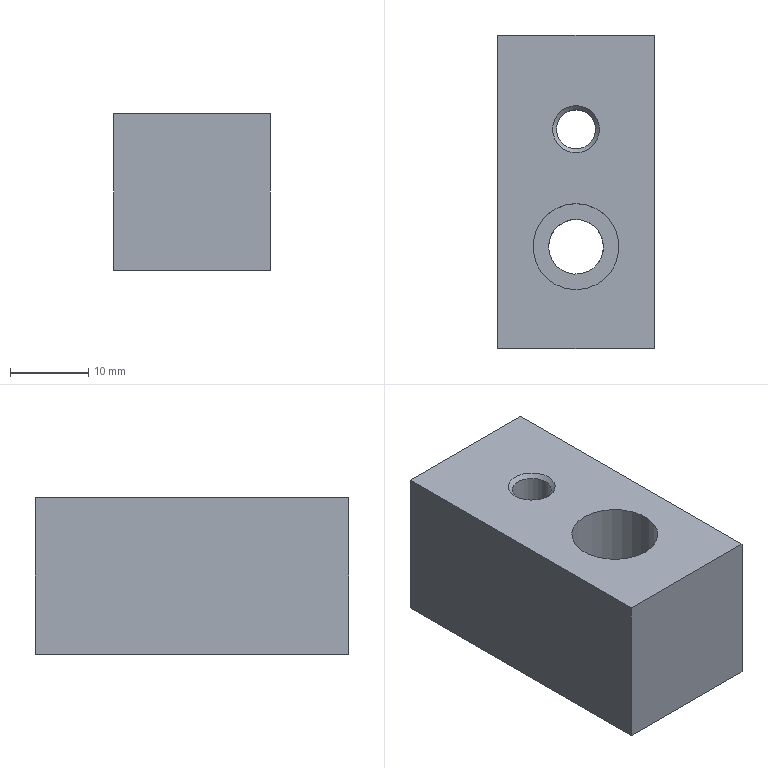Part | STEP file | gslz 2016.10.28-6_id18_x_t | 1 solid | 11 faces | box 20 x 40 x 20 mm | volume 14270 mm3 | plane 7 | cylinder 3 | cone 1 | commonest cylinder face diameters 5 x1 7 x1 11 x1
STEP:
#1=CARTESIAN_POINT('',(-127.2,158.,10.));
#2=VERTEX_POINT('',#1);
#3=CARTESIAN_POINT('',(-130.2,158.,10.));
#4=DIRECTION('',(0.,0.,-1.));
#5=DIRECTION('',(1.,0.,0.));
#6=AXIS2_PLACEMENT_3D('',#3,#4,#5);
#7=CIRCLE('',#6,3.);
#8=EDGE_CURVE('',#2,#2,#7,.T.);
#9=ORIENTED_EDGE('',*,*,#8,.T.);
#10=EDGE_LOOP('',(#9));
#11=FACE_BOUND('',#10,.T.);
#12=CARTESIAN_POINT('',(-140.2,130.,10.));
#13=VERTEX_POINT('',#12);
#14=CARTESIAN_POINT('',(-120.2,130.,10.));
#15=VERTEX_POINT('',#14);
#16=CARTESIAN_POINT('',(-138.2,130.,10.));
#17=DIRECTION('',(1.,0.,0.));
#18=VECTOR('',#17,1.);
#19=LINE('',#16,#18);
#20=EDGE_CURVE('',#13,#15,#19,.T.);
#21=ORIENTED_EDGE('',*,*,#20,.T.);
#22=CARTESIAN_POINT('',(-120.2,170.,10.));
#23=VERTEX_POINT('',#22);
#24=CARTESIAN_POINT('',(-120.2,130.,10.));
#25=DIRECTION('',(0.,1.,0.));
#26=VECTOR('',#25,1.);
#27=LINE('',#24,#26);
#28=EDGE_CURVE('',#15,#23,#27,.T.);
#29=ORIENTED_EDGE('',*,*,#28,.T.);
#30=CARTESIAN_POINT('',(-140.2,170.,10.));
#31=VERTEX_POINT('',#30);
#32=CARTESIAN_POINT('',(-122.2,170.,10.));
#33=DIRECTION('',(-1.,0.,0.));
#34=VECTOR('',#33,1.);
#35=LINE('',#32,#34);
#36=EDGE_CURVE('',#23,#31,#35,.T.);
#37=ORIENTED_EDGE('',*,*,#36,.T.);
#38=CARTESIAN_POINT('',(-140.2,160.,10.));
#39=DIRECTION('',(0.,-1.,0.));
#40=VECTOR('',#39,1.);
#41=LINE('',#38,#40);
#42=EDGE_CURVE('',#31,#13,#41,.T.);
#43=ORIENTED_EDGE('',*,*,#42,.T.);
#44=EDGE_LOOP('',(#21,#29,#37,#43));
#45=FACE_BOUND('',#44,.T.);
#46=CARTESIAN_POINT('',(-130.2,148.5,10.));
#47=VERTEX_POINT('',#46);
#48=CARTESIAN_POINT('',(-130.2,143.,10.));
#49=DIRECTION('',(0.,0.,1.));
#50=DIRECTION('',(0.,1.,0.));
#51=AXIS2_PLACEMENT_3D('',#48,#49,#50);
#52=CIRCLE('',#51,5.5);
#53=EDGE_CURVE('',#47,#47,#52,.T.);
#54=ORIENTED_EDGE('',*,*,#53,.F.);
#55=EDGE_LOOP('',(#54));
#56=FACE_BOUND('',#55,.T.);
#57=CARTESIAN_POINT('',(-138.2,130.,10.));
#58=DIRECTION('',(0.,0.,1.));
#59=DIRECTION('',(0.,-1.,0.));
#60=AXIS2_PLACEMENT_3D('',#57,#58,#59);
#61=PLANE('',#60);
#62=ADVANCED_FACE('',(#11,#45,#56),#61,.T.);
#63=CARTESIAN_POINT('',(-130.2,146.5,0.));
#64=VERTEX_POINT('',#63);
#65=CARTESIAN_POINT('',(-130.2,143.,0.));
#66=DIRECTION('',(0.,0.,1.));
#67=DIRECTION('',(0.,1.,0.));
#68=AXIS2_PLACEMENT_3D('',#65,#66,#67);
#69=CIRCLE('',#68,3.5);
#70=EDGE_CURVE('',#64,#64,#69,.T.);
#71=ORIENTED_EDGE('',*,*,#70,.F.);
#72=EDGE_LOOP('',(#71));
#73=FACE_BOUND('',#72,.T.);
#74=CARTESIAN_POINT('',(-130.2,148.5,0.));
#75=VERTEX_POINT('',#74);
#76=CARTESIAN_POINT('',(-130.2,143.,0.));
#77=DIRECTION('',(0.,0.,1.));
#78=DIRECTION('',(0.,1.,0.));
#79=AXIS2_PLACEMENT_3D('',#76,#77,#78);
#80=CIRCLE('',#79,5.5);
#81=EDGE_CURVE('',#75,#75,#80,.T.);
#82=ORIENTED_EDGE('',*,*,#81,.T.);
#83=EDGE_LOOP('',(#82));
#84=FACE_BOUND('',#83,.T.);
#85=CARTESIAN_POINT('',(-130.2,143.,0.));
#86=DIRECTION('',(0.,0.,1.));
#87=DIRECTION('',(0.,-1.,0.));
#88=AXIS2_PLACEMENT_3D('',#85,#86,#87);
#89=PLANE('',#88);
#90=ADVANCED_FACE('',(#73,#84),#89,.T.);
#91=CARTESIAN_POINT('',(-127.7,158.,9.5));
#92=VERTEX_POINT('',#91);
#93=CARTESIAN_POINT('',(-130.2,158.,9.5));
#94=DIRECTION('',(0.,0.,1.));
#95=DIRECTION('',(1.,0.,0.));
#96=AXIS2_PLACEMENT_3D('',#93,#94,#95);
#97=CIRCLE('',#96,2.5);
#98=EDGE_CURVE('',#92,#92,#97,.T.);
#99=ORIENTED_EDGE('',*,*,#98,.T.);
#100=EDGE_LOOP('',(#99));
#101=FACE_BOUND('',#100,.T.);
#102=CARTESIAN_POINT('',(-132.7,158.,-10.));
#103=VERTEX_POINT('',#102);
#104=CARTESIAN_POINT('',(-130.2,158.,-10.));
#105=DIRECTION('',(0.,0.,-1.));
#106=DIRECTION('',(-1.,0.,0.));
#107=AXIS2_PLACEMENT_3D('',#104,#105,#106);
#108=CIRCLE('',#107,2.5);
#109=EDGE_CURVE('',#103,#103,#108,.T.);
#110=ORIENTED_EDGE('',*,*,#109,.T.);
#111=EDGE_LOOP('',(#110));
#112=FACE_BOUND('',#111,.T.);
#113=CARTESIAN_POINT('',(-130.2,158.,24.));
#114=DIRECTION('',(0.,0.,-1.));
#115=DIRECTION('',(-1.,0.,0.));
#116=AXIS2_PLACEMENT_3D('',#113,#114,#115);
#117=CYLINDRICAL_SURFACE('',#116,2.5);
#118=ADVANCED_FACE('',(#101,#112),#117,.F.);
#119=ORIENTED_EDGE('',*,*,#36,.F.);
#120=CARTESIAN_POINT('',(-120.2,170.,-10.));
#121=VERTEX_POINT('',#120);
#122=CARTESIAN_POINT('',(-120.2,170.,8.));
#123=DIRECTION('',(0.,0.,1.));
#124=VECTOR('',#123,1.);
#125=LINE('',#122,#124);
#126=EDGE_CURVE('',#121,#23,#125,.T.);
#127=ORIENTED_EDGE('',*,*,#126,.F.);
#128=CARTESIAN_POINT('',(-140.2,170.,-10.));
#129=VERTEX_POINT('',#128);
#130=CARTESIAN_POINT('',(-122.2,170.,-10.));
#131=DIRECTION('',(-1.,0.,0.));
#132=VECTOR('',#131,1.);
#133=LINE('',#130,#132);
#134=EDGE_CURVE('',#121,#129,#133,.T.);
#135=ORIENTED_EDGE('',*,*,#134,.T.);
#136=CARTESIAN_POINT('',(-140.2,170.,8.));
#137=DIRECTION('',(0.,0.,1.));
#138=VECTOR('',#137,1.);
#139=LINE('',#136,#138);
#140=EDGE_CURVE('',#129,#31,#139,.T.);
#141=ORIENTED_EDGE('',*,*,#140,.T.);
#142=EDGE_LOOP('',(#119,#127,#135,#141));
#143=FACE_OUTER_BOUND('',#142,.T.);
#144=CARTESIAN_POINT('',(-122.2,170.,8.));
#145=DIRECTION('',(0.,-1.,0.));
#146=DIRECTION('',(0.,0.,-1.));
#147=AXIS2_PLACEMENT_3D('',#144,#145,#146);
#148=PLANE('',#147);
#149=ADVANCED_FACE('',(#143),#148,.F.);
#150=ORIENTED_EDGE('',*,*,#42,.F.);
#151=ORIENTED_EDGE('',*,*,#140,.F.);
#152=CARTESIAN_POINT('',(-140.2,130.,-10.));
#153=VERTEX_POINT('',#152);
#154=CARTESIAN_POINT('',(-140.2,160.,-10.));
#155=DIRECTION('',(0.,-1.,0.));
#156=VECTOR('',#155,1.);
#157=LINE('',#154,#156);
#158=EDGE_CURVE('',#129,#153,#157,.T.);
#159=ORIENTED_EDGE('',*,*,#158,.T.);
#160=CARTESIAN_POINT('',(-140.2,130.,8.));
#161=DIRECTION('',(0.,0.,1.));
#162=VECTOR('',#161,1.);
#163=LINE('',#160,#162);
#164=EDGE_CURVE('',#153,#13,#163,.T.);
#165=ORIENTED_EDGE('',*,*,#164,.T.);
#166=EDGE_LOOP('',(#150,#151,#159,#165));
#167=FACE_OUTER_BOUND('',#166,.T.);
#168=CARTESIAN_POINT('',(-140.2,160.,8.));
#169=DIRECTION('',(1.,0.,0.));
#170=DIRECTION('',(0.,0.,1.));
#171=AXIS2_PLACEMENT_3D('',#168,#169,#170);
#172=PLANE('',#171);
#173=ADVANCED_FACE('',(#167),#172,.F.);
#174=CARTESIAN_POINT('',(-120.2,130.,-10.));
#175=VERTEX_POINT('',#174);
#176=CARTESIAN_POINT('',(-138.2,130.,-10.));
#177=DIRECTION('',(1.,0.,0.));
#178=VECTOR('',#177,1.);
#179=LINE('',#176,#178);
#180=EDGE_CURVE('',#153,#175,#179,.T.);
#181=ORIENTED_EDGE('',*,*,#180,.T.);
#182=CARTESIAN_POINT('',(-120.2,130.,8.));
#183=DIRECTION('',(0.,0.,1.));
#184=VECTOR('',#183,1.);
#185=LINE('',#182,#184);
#186=EDGE_CURVE('',#175,#15,#185,.T.);
#187=ORIENTED_EDGE('',*,*,#186,.T.);
#188=ORIENTED_EDGE('',*,*,#20,.F.);
#189=ORIENTED_EDGE('',*,*,#164,.F.);
#190=EDGE_LOOP('',(#181,#187,#188,#189));
#191=FACE_OUTER_BOUND('',#190,.T.);
#192=CARTESIAN_POINT('',(-138.2,130.,8.));
#193=DIRECTION('',(0.,1.,0.));
#194=DIRECTION('',(0.,0.,1.));
#195=AXIS2_PLACEMENT_3D('',#192,#193,#194);
#196=PLANE('',#195);
#197=ADVANCED_FACE('',(#191),#196,.F.);
#198=ORIENTED_EDGE('',*,*,#28,.F.);
#199=ORIENTED_EDGE('',*,*,#186,.F.);
#200=CARTESIAN_POINT('',(-120.2,130.,-10.));
#201=DIRECTION('',(0.,1.,0.));
#202=VECTOR('',#201,1.);
#203=LINE('',#200,#202);
#204=EDGE_CURVE('',#175,#121,#203,.T.);
#205=ORIENTED_EDGE('',*,*,#204,.T.);
#206=ORIENTED_EDGE('',*,*,#126,.T.);
#207=EDGE_LOOP('',(#198,#199,#205,#206));
#208=FACE_OUTER_BOUND('',#207,.T.);
#209=CARTESIAN_POINT('',(-120.2,130.,8.));
#210=DIRECTION('',(-1.,0.,0.));
#211=DIRECTION('',(0.,0.,-1.));
#212=AXIS2_PLACEMENT_3D('',#209,#210,#211);
#213=PLANE('',#212);
#214=ADVANCED_FACE('',(#208),#213,.F.);
#215=CARTESIAN_POINT('',(-133.7,143.,-10.));
#216=VERTEX_POINT('',#215);
#217=CARTESIAN_POINT('',(-130.2,143.,-10.));
#218=DIRECTION('',(0.,0.,-1.));
#219=DIRECTION('',(-1.,0.,0.));
#220=AXIS2_PLACEMENT_3D('',#217,#218,#219);
#221=CIRCLE('',#220,3.5);
#222=EDGE_CURVE('',#216,#216,#221,.T.);
#223=ORIENTED_EDGE('',*,*,#222,.T.);
#224=EDGE_LOOP('',(#223));
#225=FACE_BOUND('',#224,.T.);
#226=ORIENTED_EDGE('',*,*,#70,.T.);
#227=EDGE_LOOP('',(#226));
#228=FACE_BOUND('',#227,.T.);
#229=CARTESIAN_POINT('',(-130.2,143.,24.));
#230=DIRECTION('',(0.,0.,-1.));
#231=DIRECTION('',(-1.,0.,0.));
#232=AXIS2_PLACEMENT_3D('',#229,#230,#231);
#233=CYLINDRICAL_SURFACE('',#232,3.5);
#234=ADVANCED_FACE('',(#225,#228),#233,.F.);
#235=ORIENTED_EDGE('',*,*,#222,.F.);
#236=EDGE_LOOP('',(#235));
#237=FACE_BOUND('',#236,.T.);
#238=ORIENTED_EDGE('',*,*,#204,.F.);
#239=ORIENTED_EDGE('',*,*,#180,.F.);
#240=ORIENTED_EDGE('',*,*,#158,.F.);
#241=ORIENTED_EDGE('',*,*,#134,.F.);
#242=EDGE_LOOP('',(#238,#239,#240,#241));
#243=FACE_BOUND('',#242,.T.);
#244=ORIENTED_EDGE('',*,*,#109,.F.);
#245=EDGE_LOOP('',(#244));
#246=FACE_BOUND('',#245,.T.);
#247=CARTESIAN_POINT('',(-130.2,130.,-10.));
#248=DIRECTION('',(0.,0.,-1.));
#249=DIRECTION('',(0.,1.,0.));
#250=AXIS2_PLACEMENT_3D('',#247,#248,#249);
#251=PLANE('',#250);
#252=ADVANCED_FACE('',(#237,#243,#246),#251,.T.);
#253=ORIENTED_EDGE('',*,*,#81,.F.);
#254=EDGE_LOOP('',(#253));
#255=FACE_BOUND('',#254,.T.);
#256=ORIENTED_EDGE('',*,*,#53,.T.);
#257=EDGE_LOOP('',(#256));
#258=FACE_BOUND('',#257,.T.);
#259=CARTESIAN_POINT('',(-130.2,143.,0.));
#260=DIRECTION('',(0.,0.,1.));
#261=DIRECTION('',(1.,0.,0.));
#262=AXIS2_PLACEMENT_3D('',#259,#260,#261);
#263=CYLINDRICAL_SURFACE('',#262,5.5);
#264=ADVANCED_FACE('',(#255,#258),#263,.F.);
#265=ORIENTED_EDGE('',*,*,#98,.F.);
#266=EDGE_LOOP('',(#265));
#267=FACE_BOUND('',#266,.T.);
#268=ORIENTED_EDGE('',*,*,#8,.F.);
#269=EDGE_LOOP('',(#268));
#270=FACE_BOUND('',#269,.T.);
#271=CARTESIAN_POINT('',(-130.2,158.,10.));
#272=DIRECTION('',(0.,0.,1.));
#273=DIRECTION('',(1.,0.,0.));
#274=AXIS2_PLACEMENT_3D('',#271,#272,#273);
#275=CONICAL_SURFACE('',#274,3.,45.);
#276=ADVANCED_FACE('',(#267,#270),#275,.F.);
#277=CLOSED_SHELL('',(#62,#90,#118,#149,#173,#197,#214,#234,#252,#264,#276));
#278=MANIFOLD_SOLID_BREP('',#277);
#279=(LENGTH_UNIT()NAMED_UNIT(*)SI_UNIT(.MILLI.,.METRE.));
#280=UNCERTAINTY_MEASURE_WITH_UNIT(LENGTH_MEASURE(0.00002),#279,'','');
#281=(NAMED_UNIT(*)PLANE_ANGLE_UNIT()SI_UNIT($,.RADIAN.));
#282=PLANE_ANGLE_MEASURE_WITH_UNIT(PLANE_ANGLE_MEASURE(0.01745),#281);
#283=DIMENSIONAL_EXPONENTS(0.,0.,0.,0.,0.,0.,0.);
#284=(CONVERSION_BASED_UNIT('DEGREE',#282)NAMED_UNIT(#283)PLANE_ANGLE_UNIT());
#285=(NAMED_UNIT(*)SI_UNIT($,.STERADIAN.)SOLID_ANGLE_UNIT());
#286=(GEOMETRIC_REPRESENTATION_CONTEXT(3)GLOBAL_UNCERTAINTY_ASSIGNED_CONTEXT((#280))GLOBAL_UNIT_ASSIGNED_CONTEXT((#279,#284,#285))REPRESENTATION_CONTEXT('',''));
#287=ADVANCED_BREP_SHAPE_REPRESENTATION('',(#278),#286);